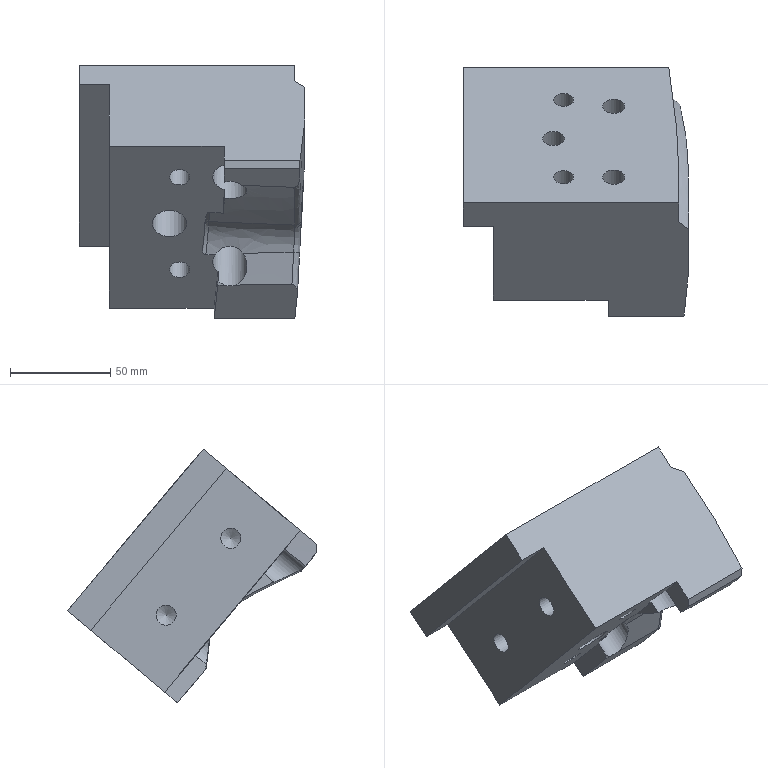Part | NX | features MAIN_BODY 2 | 1 solid | 48 faces | box 112.313 x 123.827 x 126.301 mm | volume 621192 mm3 | spline 25 | plane 11 | cylinder 10 | cone 2 | commonest cylinder face diameters 10 x4 11 x3 17 x3